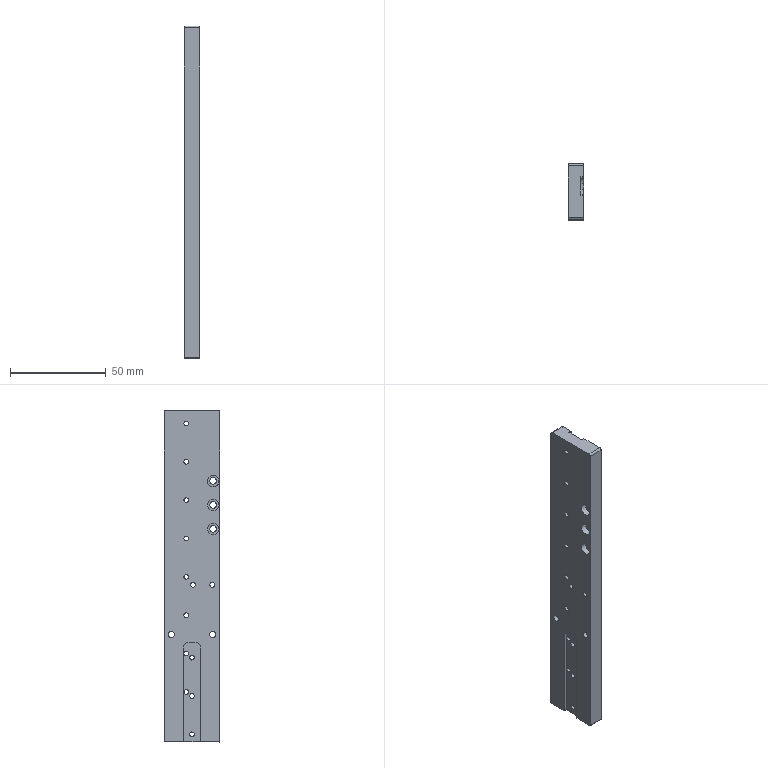Part | 1 solid | 55 faces | box 8 x 29 x 173.1 mm | volume 36196 mm3 | cylinder 29 | plane 26 | commonest cylinder face diameters 2.5 x13 3.3 x4 6.07 x4 3.5 x3 6 x3 2 x2